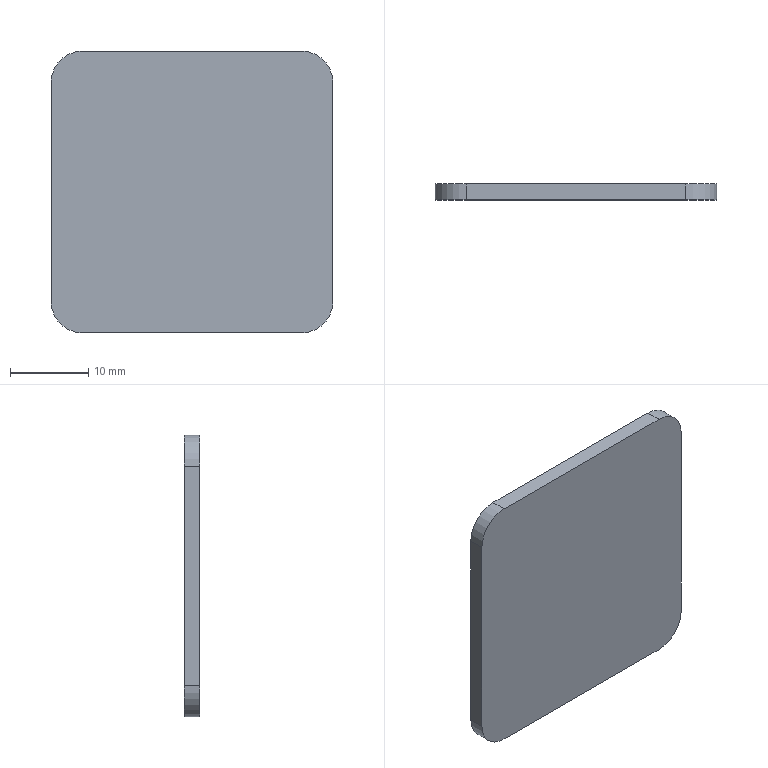Part | SolidWorks | features Extrusion 1, Fillet 1 | 1 solid | 10 faces | box 36 x 2 x 36 mm | volume 2565 mm3 | plane 6 | cylinder 4 | commonest cylinder face diameters 8 x4
STEP:
#1=CARTESIAN_POINT('',(18.,1.,14.));
#2=VERTEX_POINT('',#1);
#3=CARTESIAN_POINT('',(18.,1.,-14.));
#4=VERTEX_POINT('',#3);
#5=CARTESIAN_POINT('',(18.,1.,-18.));
#6=DIRECTION('',(0.,0.,-1.));
#7=VECTOR('',#6,1000.);
#8=LINE('',#5,#7);
#9=EDGE_CURVE('',#2,#4,#8,.T.);
#10=ORIENTED_EDGE('',*,*,#9,.F.);
#11=CARTESIAN_POINT('',(18.,-1.,14.));
#12=VERTEX_POINT('',#11);
#13=CARTESIAN_POINT('',(18.,1.,14.));
#14=DIRECTION('',(0.,-1.,0.));
#15=VECTOR('',#14,1000.);
#16=LINE('',#13,#15);
#17=EDGE_CURVE('',#2,#12,#16,.T.);
#18=ORIENTED_EDGE('',*,*,#17,.T.);
#19=CARTESIAN_POINT('',(18.,-1.,-14.));
#20=VERTEX_POINT('',#19);
#21=CARTESIAN_POINT('',(18.,-1.,-18.));
#22=DIRECTION('',(0.,0.,-1.));
#23=VECTOR('',#22,1000.);
#24=LINE('',#21,#23);
#25=EDGE_CURVE('',#12,#20,#24,.T.);
#26=ORIENTED_EDGE('',*,*,#25,.T.);
#27=CARTESIAN_POINT('',(18.,1.,-14.));
#28=DIRECTION('',(0.,1.,0.));
#29=VECTOR('',#28,1000.);
#30=LINE('',#27,#29);
#31=EDGE_CURVE('',#20,#4,#30,.T.);
#32=ORIENTED_EDGE('',*,*,#31,.T.);
#33=EDGE_LOOP('',(#10,#18,#26,#32));
#34=FACE_OUTER_BOUND('',#33,.T.);
#35=CARTESIAN_POINT('',(18.,1.,-18.));
#36=DIRECTION('',(-1.,0.,0.));
#37=DIRECTION('',(0.,0.,1.));
#38=AXIS2_PLACEMENT_3D('',#35,#36,#37);
#39=PLANE('',#38);
#40=ADVANCED_FACE('',(#34),#39,.F.);
#41=CARTESIAN_POINT('',(14.,1.,-18.));
#42=VERTEX_POINT('',#41);
#43=CARTESIAN_POINT('',(-14.,1.,-18.));
#44=VERTEX_POINT('',#43);
#45=CARTESIAN_POINT('',(-18.,1.,-18.));
#46=DIRECTION('',(-1.,0.,0.));
#47=VECTOR('',#46,1000.);
#48=LINE('',#45,#47);
#49=EDGE_CURVE('',#42,#44,#48,.T.);
#50=ORIENTED_EDGE('',*,*,#49,.F.);
#51=CARTESIAN_POINT('',(14.,-1.,-18.));
#52=VERTEX_POINT('',#51);
#53=CARTESIAN_POINT('',(14.,1.,-18.));
#54=DIRECTION('',(0.,-1.,0.));
#55=VECTOR('',#54,1000.);
#56=LINE('',#53,#55);
#57=EDGE_CURVE('',#42,#52,#56,.T.);
#58=ORIENTED_EDGE('',*,*,#57,.T.);
#59=CARTESIAN_POINT('',(-14.,-1.,-18.));
#60=VERTEX_POINT('',#59);
#61=CARTESIAN_POINT('',(-18.,-1.,-18.));
#62=DIRECTION('',(-1.,0.,0.));
#63=VECTOR('',#62,1000.);
#64=LINE('',#61,#63);
#65=EDGE_CURVE('',#52,#60,#64,.T.);
#66=ORIENTED_EDGE('',*,*,#65,.T.);
#67=CARTESIAN_POINT('',(-14.,1.,-18.));
#68=DIRECTION('',(0.,1.,0.));
#69=VECTOR('',#68,1000.);
#70=LINE('',#67,#69);
#71=EDGE_CURVE('',#60,#44,#70,.T.);
#72=ORIENTED_EDGE('',*,*,#71,.T.);
#73=EDGE_LOOP('',(#50,#58,#66,#72));
#74=FACE_OUTER_BOUND('',#73,.T.);
#75=CARTESIAN_POINT('',(-18.,1.,-18.));
#76=DIRECTION('',(0.,0.,1.));
#77=DIRECTION('',(1.,0.,0.));
#78=AXIS2_PLACEMENT_3D('',#75,#76,#77);
#79=PLANE('',#78);
#80=ADVANCED_FACE('',(#74),#79,.F.);
#81=CARTESIAN_POINT('',(-18.,-1.,-14.));
#82=VERTEX_POINT('',#81);
#83=CARTESIAN_POINT('',(-18.,-1.,14.));
#84=VERTEX_POINT('',#83);
#85=CARTESIAN_POINT('',(-18.,-1.,-18.));
#86=DIRECTION('',(0.,0.,1.));
#87=VECTOR('',#86,1000.);
#88=LINE('',#85,#87);
#89=EDGE_CURVE('',#82,#84,#88,.T.);
#90=ORIENTED_EDGE('',*,*,#89,.T.);
#91=CARTESIAN_POINT('',(-18.,1.,14.));
#92=VERTEX_POINT('',#91);
#93=CARTESIAN_POINT('',(-18.,1.,14.));
#94=DIRECTION('',(0.,1.,0.));
#95=VECTOR('',#94,1000.);
#96=LINE('',#93,#95);
#97=EDGE_CURVE('',#84,#92,#96,.T.);
#98=ORIENTED_EDGE('',*,*,#97,.T.);
#99=CARTESIAN_POINT('',(-18.,1.,-14.));
#100=VERTEX_POINT('',#99);
#101=CARTESIAN_POINT('',(-18.,1.,-18.));
#102=DIRECTION('',(0.,0.,1.));
#103=VECTOR('',#102,1000.);
#104=LINE('',#101,#103);
#105=EDGE_CURVE('',#100,#92,#104,.T.);
#106=ORIENTED_EDGE('',*,*,#105,.F.);
#107=CARTESIAN_POINT('',(-18.,1.,-14.));
#108=DIRECTION('',(0.,-1.,0.));
#109=VECTOR('',#108,1000.);
#110=LINE('',#107,#109);
#111=EDGE_CURVE('',#100,#82,#110,.T.);
#112=ORIENTED_EDGE('',*,*,#111,.T.);
#113=EDGE_LOOP('',(#90,#98,#106,#112));
#114=FACE_OUTER_BOUND('',#113,.T.);
#115=CARTESIAN_POINT('',(-18.,1.,-18.));
#116=DIRECTION('',(1.,0.,0.));
#117=DIRECTION('',(0.,0.,-1.));
#118=AXIS2_PLACEMENT_3D('',#115,#116,#117);
#119=PLANE('',#118);
#120=ADVANCED_FACE('',(#114),#119,.F.);
#121=CARTESIAN_POINT('',(-14.,1.,18.));
#122=VERTEX_POINT('',#121);
#123=CARTESIAN_POINT('',(14.,1.,18.));
#124=VERTEX_POINT('',#123);
#125=CARTESIAN_POINT('',(-18.,1.,18.));
#126=DIRECTION('',(1.,0.,0.));
#127=VECTOR('',#126,1000.);
#128=LINE('',#125,#127);
#129=EDGE_CURVE('',#122,#124,#128,.T.);
#130=ORIENTED_EDGE('',*,*,#129,.F.);
#131=CARTESIAN_POINT('',(-14.,-1.,18.));
#132=VERTEX_POINT('',#131);
#133=CARTESIAN_POINT('',(-14.,1.,18.));
#134=DIRECTION('',(0.,-1.,0.));
#135=VECTOR('',#134,1000.);
#136=LINE('',#133,#135);
#137=EDGE_CURVE('',#122,#132,#136,.T.);
#138=ORIENTED_EDGE('',*,*,#137,.T.);
#139=CARTESIAN_POINT('',(14.,-1.,18.));
#140=VERTEX_POINT('',#139);
#141=CARTESIAN_POINT('',(-18.,-1.,18.));
#142=DIRECTION('',(1.,0.,0.));
#143=VECTOR('',#142,1000.);
#144=LINE('',#141,#143);
#145=EDGE_CURVE('',#132,#140,#144,.T.);
#146=ORIENTED_EDGE('',*,*,#145,.T.);
#147=CARTESIAN_POINT('',(14.,1.,18.));
#148=DIRECTION('',(0.,1.,0.));
#149=VECTOR('',#148,1000.);
#150=LINE('',#147,#149);
#151=EDGE_CURVE('',#140,#124,#150,.T.);
#152=ORIENTED_EDGE('',*,*,#151,.T.);
#153=EDGE_LOOP('',(#130,#138,#146,#152));
#154=FACE_OUTER_BOUND('',#153,.T.);
#155=CARTESIAN_POINT('',(-18.,1.,18.));
#156=DIRECTION('',(0.,0.,-1.));
#157=DIRECTION('',(-1.,0.,0.));
#158=AXIS2_PLACEMENT_3D('',#155,#156,#157);
#159=PLANE('',#158);
#160=ADVANCED_FACE('',(#154),#159,.F.);
#161=ORIENTED_EDGE('',*,*,#105,.T.);
#162=CARTESIAN_POINT('',(-14.,1.,14.));
#163=DIRECTION('',(0.,1.,0.));
#164=DIRECTION('',(0.,0.,1.));
#165=AXIS2_PLACEMENT_3D('',#162,#163,#164);
#166=CIRCLE('',#165,4.);
#167=EDGE_CURVE('',#92,#122,#166,.T.);
#168=ORIENTED_EDGE('',*,*,#167,.T.);
#169=ORIENTED_EDGE('',*,*,#129,.T.);
#170=CARTESIAN_POINT('',(14.,1.,14.));
#171=DIRECTION('',(0.,1.,0.));
#172=DIRECTION('',(0.,0.,1.));
#173=AXIS2_PLACEMENT_3D('',#170,#171,#172);
#174=CIRCLE('',#173,4.);
#175=EDGE_CURVE('',#124,#2,#174,.T.);
#176=ORIENTED_EDGE('',*,*,#175,.T.);
#177=ORIENTED_EDGE('',*,*,#9,.T.);
#178=CARTESIAN_POINT('',(14.,1.,-14.));
#179=DIRECTION('',(0.,1.,0.));
#180=DIRECTION('',(0.,0.,1.));
#181=AXIS2_PLACEMENT_3D('',#178,#179,#180);
#182=CIRCLE('',#181,4.);
#183=EDGE_CURVE('',#4,#42,#182,.T.);
#184=ORIENTED_EDGE('',*,*,#183,.T.);
#185=ORIENTED_EDGE('',*,*,#49,.T.);
#186=CARTESIAN_POINT('',(-14.,1.,-14.));
#187=DIRECTION('',(0.,1.,0.));
#188=DIRECTION('',(0.,0.,1.));
#189=AXIS2_PLACEMENT_3D('',#186,#187,#188);
#190=CIRCLE('',#189,4.);
#191=EDGE_CURVE('',#44,#100,#190,.T.);
#192=ORIENTED_EDGE('',*,*,#191,.T.);
#193=EDGE_LOOP('',(#161,#168,#169,#176,#177,#184,#185,#192));
#194=FACE_OUTER_BOUND('',#193,.T.);
#195=CARTESIAN_POINT('',(0.,1.,0.));
#196=DIRECTION('',(0.,1.,0.));
#197=DIRECTION('',(0.,0.,1.));
#198=AXIS2_PLACEMENT_3D('',#195,#196,#197);
#199=PLANE('',#198);
#200=ADVANCED_FACE('',(#194),#199,.T.);
#201=ORIENTED_EDGE('',*,*,#145,.F.);
#202=CARTESIAN_POINT('',(-14.,-1.,14.));
#203=DIRECTION('',(0.,-1.,0.));
#204=DIRECTION('',(0.,0.,1.));
#205=AXIS2_PLACEMENT_3D('',#202,#203,#204);
#206=CIRCLE('',#205,4.);
#207=EDGE_CURVE('',#132,#84,#206,.T.);
#208=ORIENTED_EDGE('',*,*,#207,.T.);
#209=ORIENTED_EDGE('',*,*,#89,.F.);
#210=CARTESIAN_POINT('',(-14.,-1.,-14.));
#211=DIRECTION('',(0.,-1.,0.));
#212=DIRECTION('',(0.,0.,1.));
#213=AXIS2_PLACEMENT_3D('',#210,#211,#212);
#214=CIRCLE('',#213,4.);
#215=EDGE_CURVE('',#82,#60,#214,.T.);
#216=ORIENTED_EDGE('',*,*,#215,.T.);
#217=ORIENTED_EDGE('',*,*,#65,.F.);
#218=CARTESIAN_POINT('',(14.,-1.,-14.));
#219=DIRECTION('',(0.,-1.,0.));
#220=DIRECTION('',(0.,0.,1.));
#221=AXIS2_PLACEMENT_3D('',#218,#219,#220);
#222=CIRCLE('',#221,4.);
#223=EDGE_CURVE('',#52,#20,#222,.T.);
#224=ORIENTED_EDGE('',*,*,#223,.T.);
#225=ORIENTED_EDGE('',*,*,#25,.F.);
#226=CARTESIAN_POINT('',(14.,-1.,14.));
#227=DIRECTION('',(0.,-1.,0.));
#228=DIRECTION('',(0.,0.,1.));
#229=AXIS2_PLACEMENT_3D('',#226,#227,#228);
#230=CIRCLE('',#229,4.);
#231=EDGE_CURVE('',#12,#140,#230,.T.);
#232=ORIENTED_EDGE('',*,*,#231,.T.);
#233=EDGE_LOOP('',(#201,#208,#209,#216,#217,#224,#225,#232));
#234=FACE_OUTER_BOUND('',#233,.T.);
#235=CARTESIAN_POINT('',(0.,-1.,0.));
#236=DIRECTION('',(0.,1.,0.));
#237=DIRECTION('',(0.,0.,1.));
#238=AXIS2_PLACEMENT_3D('',#235,#236,#237);
#239=PLANE('',#238);
#240=ADVANCED_FACE('',(#234),#239,.F.);
#241=ORIENTED_EDGE('',*,*,#167,.F.);
#242=ORIENTED_EDGE('',*,*,#97,.F.);
#243=ORIENTED_EDGE('',*,*,#207,.F.);
#244=ORIENTED_EDGE('',*,*,#137,.F.);
#245=EDGE_LOOP('',(#241,#242,#243,#244));
#246=FACE_OUTER_BOUND('',#245,.T.);
#247=CARTESIAN_POINT('',(-14.,1.,14.));
#248=DIRECTION('',(0.,-1.,0.));
#249=DIRECTION('',(0.,0.,-1.));
#250=AXIS2_PLACEMENT_3D('',#247,#248,#249);
#251=CYLINDRICAL_SURFACE('',#250,4.);
#252=ADVANCED_FACE('',(#246),#251,.T.);
#253=ORIENTED_EDGE('',*,*,#175,.F.);
#254=ORIENTED_EDGE('',*,*,#151,.F.);
#255=ORIENTED_EDGE('',*,*,#231,.F.);
#256=ORIENTED_EDGE('',*,*,#17,.F.);
#257=EDGE_LOOP('',(#253,#254,#255,#256));
#258=FACE_OUTER_BOUND('',#257,.T.);
#259=CARTESIAN_POINT('',(14.,1.,14.));
#260=DIRECTION('',(0.,-1.,0.));
#261=DIRECTION('',(0.,0.,-1.));
#262=AXIS2_PLACEMENT_3D('',#259,#260,#261);
#263=CYLINDRICAL_SURFACE('',#262,4.);
#264=ADVANCED_FACE('',(#258),#263,.T.);
#265=ORIENTED_EDGE('',*,*,#183,.F.);
#266=ORIENTED_EDGE('',*,*,#31,.F.);
#267=ORIENTED_EDGE('',*,*,#223,.F.);
#268=ORIENTED_EDGE('',*,*,#57,.F.);
#269=EDGE_LOOP('',(#265,#266,#267,#268));
#270=FACE_OUTER_BOUND('',#269,.T.);
#271=CARTESIAN_POINT('',(14.,1.,-14.));
#272=DIRECTION('',(0.,-1.,0.));
#273=DIRECTION('',(0.,0.,-1.));
#274=AXIS2_PLACEMENT_3D('',#271,#272,#273);
#275=CYLINDRICAL_SURFACE('',#274,4.);
#276=ADVANCED_FACE('',(#270),#275,.T.);
#277=ORIENTED_EDGE('',*,*,#191,.F.);
#278=ORIENTED_EDGE('',*,*,#71,.F.);
#279=ORIENTED_EDGE('',*,*,#215,.F.);
#280=ORIENTED_EDGE('',*,*,#111,.F.);
#281=EDGE_LOOP('',(#277,#278,#279,#280));
#282=FACE_OUTER_BOUND('',#281,.T.);
#283=CARTESIAN_POINT('',(-14.,1.,-14.));
#284=DIRECTION('',(0.,-1.,0.));
#285=DIRECTION('',(0.,0.,-1.));
#286=AXIS2_PLACEMENT_3D('',#283,#284,#285);
#287=CYLINDRICAL_SURFACE('',#286,4.);
#288=ADVANCED_FACE('',(#282),#287,.T.);
#289=CLOSED_SHELL('',(#40,#80,#120,#160,#200,#240,#252,#264,#276,#288));
#290=MANIFOLD_SOLID_BREP('',#289);
#291=CARTESIAN_POINT('',(0.,0.,0.));
#292=DIRECTION('',(0.,0.,1.));
#293=DIRECTION('',(1.,0.,0.));
#294=AXIS2_PLACEMENT_3D('',#291,#292,#293);
#295=(LENGTH_UNIT()NAMED_UNIT(*)SI_UNIT(.MILLI.,.METRE.));
#296=UNCERTAINTY_MEASURE_WITH_UNIT(LENGTH_MEASURE(0.00001),#295,'','');
#297=(NAMED_UNIT(*)PLANE_ANGLE_UNIT()SI_UNIT($,.RADIAN.));
#298=(NAMED_UNIT(*)SI_UNIT($,.STERADIAN.)SOLID_ANGLE_UNIT());
#299=(GEOMETRIC_REPRESENTATION_CONTEXT(3)GLOBAL_UNCERTAINTY_ASSIGNED_CONTEXT((#296))GLOBAL_UNIT_ASSIGNED_CONTEXT((#295,#297,#298))REPRESENTATION_CONTEXT('',''));
#300=ADVANCED_BREP_SHAPE_REPRESENTATION('',(#290,#294),#299);